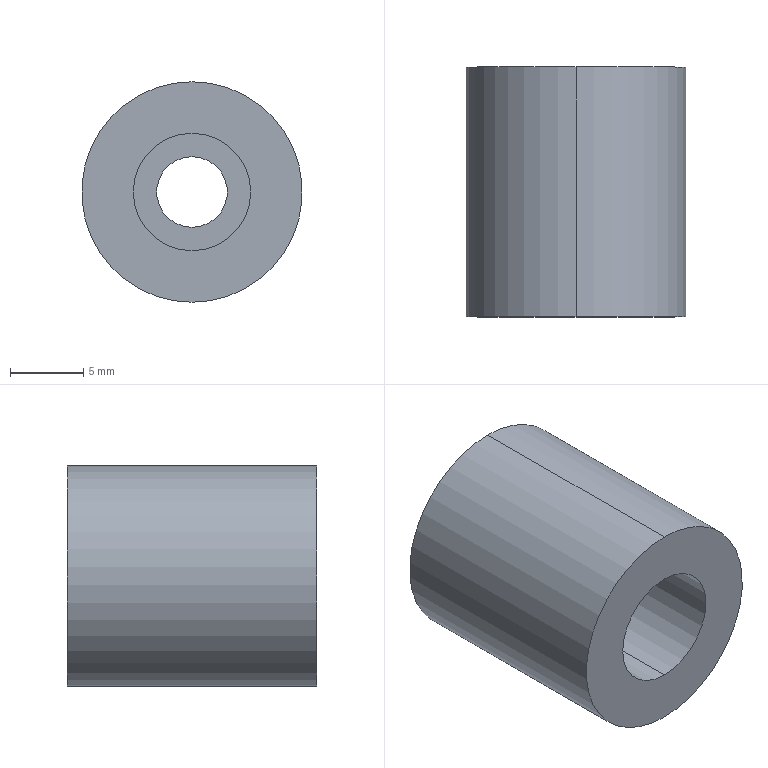Part | SolidWorks | features BaseBody 1 | 1 solid | 9 faces | box 15 x 17 x 15 mm | volume 2439 mm3 | cylinder 6 | plane 3 | commonest cylinder face diameters 4.8 x2 8 x2 15 x2
STEP:
#1=CARTESIAN_POINT('',(0.,17.,-7.5));
#2=VERTEX_POINT('',#1);
#3=CARTESIAN_POINT('',(0.,17.,7.5));
#4=VERTEX_POINT('',#3);
#5=CARTESIAN_POINT('',(0.,17.,0.));
#6=DIRECTION('',(0.,-1.,0.));
#7=DIRECTION('',(0.,0.,-1.));
#8=AXIS2_PLACEMENT_3D('',#5,#6,#7);
#9=CIRCLE('',#8,7.5);
#10=EDGE_CURVE('',#2,#4,#9,.T.);
#11=ORIENTED_EDGE('',*,*,#10,.T.);
#12=CARTESIAN_POINT('',(0.,0.,7.5));
#13=VERTEX_POINT('',#12);
#14=CARTESIAN_POINT('',(0.,17.,7.5));
#15=DIRECTION('',(0.,-1.,0.));
#16=VECTOR('',#15,1000.);
#17=LINE('',#14,#16);
#18=EDGE_CURVE('',#4,#13,#17,.T.);
#19=ORIENTED_EDGE('',*,*,#18,.T.);
#20=CARTESIAN_POINT('',(0.,0.,-7.5));
#21=VERTEX_POINT('',#20);
#22=CARTESIAN_POINT('',(0.,0.,0.));
#23=DIRECTION('',(0.,1.,0.));
#24=DIRECTION('',(0.,0.,-1.));
#25=AXIS2_PLACEMENT_3D('',#22,#23,#24);
#26=CIRCLE('',#25,7.5);
#27=EDGE_CURVE('',#13,#21,#26,.T.);
#28=ORIENTED_EDGE('',*,*,#27,.T.);
#29=CARTESIAN_POINT('',(0.,17.,-7.5));
#30=DIRECTION('',(0.,-1.,0.));
#31=VECTOR('',#30,1000.);
#32=LINE('',#29,#31);
#33=EDGE_CURVE('',#2,#21,#32,.T.);
#34=ORIENTED_EDGE('',*,*,#33,.F.);
#35=EDGE_LOOP('',(#11,#19,#28,#34));
#36=FACE_OUTER_BOUND('',#35,.T.);
#37=CARTESIAN_POINT('',(0.,17.,0.));
#38=DIRECTION('',(0.,-1.,0.));
#39=DIRECTION('',(0.,0.,-1.));
#40=AXIS2_PLACEMENT_3D('',#37,#38,#39);
#41=CYLINDRICAL_SURFACE('',#40,7.5);
#42=ADVANCED_FACE('',(#36),#41,.T.);
#43=CARTESIAN_POINT('',(0.,8.,4.));
#44=VERTEX_POINT('',#43);
#45=CARTESIAN_POINT('',(0.,8.,-4.));
#46=VERTEX_POINT('',#45);
#47=CARTESIAN_POINT('',(0.,8.,0.));
#48=DIRECTION('',(0.,-1.,0.));
#49=DIRECTION('',(0.,0.,-1.));
#50=AXIS2_PLACEMENT_3D('',#47,#48,#49);
#51=CIRCLE('',#50,4.);
#52=EDGE_CURVE('',#44,#46,#51,.T.);
#53=ORIENTED_EDGE('',*,*,#52,.F.);
#54=CARTESIAN_POINT('',(0.,0.,4.));
#55=VERTEX_POINT('',#54);
#56=CARTESIAN_POINT('',(0.,0.,4.));
#57=DIRECTION('',(0.,-1.,0.));
#58=VECTOR('',#57,1000.);
#59=LINE('',#56,#58);
#60=EDGE_CURVE('',#44,#55,#59,.T.);
#61=ORIENTED_EDGE('',*,*,#60,.T.);
#62=CARTESIAN_POINT('',(0.,0.,-4.));
#63=VERTEX_POINT('',#62);
#64=CARTESIAN_POINT('',(0.,0.,0.));
#65=DIRECTION('',(0.,-1.,0.));
#66=DIRECTION('',(0.,0.,-1.));
#67=AXIS2_PLACEMENT_3D('',#64,#65,#66);
#68=CIRCLE('',#67,4.);
#69=EDGE_CURVE('',#55,#63,#68,.T.);
#70=ORIENTED_EDGE('',*,*,#69,.T.);
#71=CARTESIAN_POINT('',(0.,0.,-4.));
#72=DIRECTION('',(0.,-1.,0.));
#73=VECTOR('',#72,1000.);
#74=LINE('',#71,#73);
#75=EDGE_CURVE('',#46,#63,#74,.T.);
#76=ORIENTED_EDGE('',*,*,#75,.F.);
#77=EDGE_LOOP('',(#53,#61,#70,#76));
#78=FACE_OUTER_BOUND('',#77,.T.);
#79=CARTESIAN_POINT('',(0.,0.,0.));
#80=DIRECTION('',(0.,-1.,0.));
#81=DIRECTION('',(0.,0.,-1.));
#82=AXIS2_PLACEMENT_3D('',#79,#80,#81);
#83=CYLINDRICAL_SURFACE('',#82,4.);
#84=ADVANCED_FACE('',(#78),#83,.F.);
#85=CARTESIAN_POINT('',(0.,17.,2.4));
#86=VERTEX_POINT('',#85);
#87=CARTESIAN_POINT('',(0.,17.,-2.4));
#88=VERTEX_POINT('',#87);
#89=CARTESIAN_POINT('',(0.,17.,0.));
#90=DIRECTION('',(0.,-1.,0.));
#91=DIRECTION('',(0.,0.,-1.));
#92=AXIS2_PLACEMENT_3D('',#89,#90,#91);
#93=CIRCLE('',#92,2.4);
#94=EDGE_CURVE('',#86,#88,#93,.T.);
#95=ORIENTED_EDGE('',*,*,#94,.F.);
#96=CARTESIAN_POINT('',(0.,8.,2.4));
#97=VERTEX_POINT('',#96);
#98=CARTESIAN_POINT('',(0.,0.,2.4));
#99=DIRECTION('',(0.,-1.,0.));
#100=VECTOR('',#99,1000.);
#101=LINE('',#98,#100);
#102=EDGE_CURVE('',#86,#97,#101,.T.);
#103=ORIENTED_EDGE('',*,*,#102,.T.);
#104=CARTESIAN_POINT('',(0.,8.,-2.4));
#105=VERTEX_POINT('',#104);
#106=CARTESIAN_POINT('',(0.,8.,0.));
#107=DIRECTION('',(0.,1.,0.));
#108=DIRECTION('',(0.,0.,-1.));
#109=AXIS2_PLACEMENT_3D('',#106,#107,#108);
#110=CIRCLE('',#109,2.4);
#111=EDGE_CURVE('',#105,#97,#110,.T.);
#112=ORIENTED_EDGE('',*,*,#111,.F.);
#113=CARTESIAN_POINT('',(0.,0.,-2.4));
#114=DIRECTION('',(0.,-1.,0.));
#115=VECTOR('',#114,1000.);
#116=LINE('',#113,#115);
#117=EDGE_CURVE('',#88,#105,#116,.T.);
#118=ORIENTED_EDGE('',*,*,#117,.F.);
#119=EDGE_LOOP('',(#95,#103,#112,#118));
#120=FACE_OUTER_BOUND('',#119,.T.);
#121=CARTESIAN_POINT('',(0.,0.,0.));
#122=DIRECTION('',(0.,-1.,0.));
#123=DIRECTION('',(0.,0.,-1.));
#124=AXIS2_PLACEMENT_3D('',#121,#122,#123);
#125=CYLINDRICAL_SURFACE('',#124,2.4);
#126=ADVANCED_FACE('',(#120),#125,.F.);
#127=ORIENTED_EDGE('',*,*,#18,.F.);
#128=CARTESIAN_POINT('',(0.,17.,0.));
#129=DIRECTION('',(0.,-1.,0.));
#130=DIRECTION('',(0.,0.,-1.));
#131=AXIS2_PLACEMENT_3D('',#128,#129,#130);
#132=CIRCLE('',#131,7.5);
#133=EDGE_CURVE('',#4,#2,#132,.T.);
#134=ORIENTED_EDGE('',*,*,#133,.T.);
#135=ORIENTED_EDGE('',*,*,#33,.T.);
#136=CARTESIAN_POINT('',(0.,0.,0.));
#137=DIRECTION('',(0.,1.,0.));
#138=DIRECTION('',(0.,0.,-1.));
#139=AXIS2_PLACEMENT_3D('',#136,#137,#138);
#140=CIRCLE('',#139,7.5);
#141=EDGE_CURVE('',#21,#13,#140,.T.);
#142=ORIENTED_EDGE('',*,*,#141,.T.);
#143=EDGE_LOOP('',(#127,#134,#135,#142));
#144=FACE_OUTER_BOUND('',#143,.T.);
#145=CARTESIAN_POINT('',(0.,17.,0.));
#146=DIRECTION('',(0.,-1.,0.));
#147=DIRECTION('',(0.,0.,-1.));
#148=AXIS2_PLACEMENT_3D('',#145,#146,#147);
#149=CYLINDRICAL_SURFACE('',#148,7.5);
#150=ADVANCED_FACE('',(#144),#149,.T.);
#151=ORIENTED_EDGE('',*,*,#141,.F.);
#152=ORIENTED_EDGE('',*,*,#27,.F.);
#153=EDGE_LOOP('',(#151,#152));
#154=FACE_OUTER_BOUND('',#153,.T.);
#155=CARTESIAN_POINT('',(0.,0.,0.));
#156=DIRECTION('',(0.,-1.,0.));
#157=DIRECTION('',(0.,0.,-1.));
#158=AXIS2_PLACEMENT_3D('',#155,#156,#157);
#159=CIRCLE('',#158,4.);
#160=EDGE_CURVE('',#63,#55,#159,.T.);
#161=ORIENTED_EDGE('',*,*,#160,.F.);
#162=ORIENTED_EDGE('',*,*,#69,.F.);
#163=EDGE_LOOP('',(#161,#162));
#164=FACE_BOUND('',#163,.T.);
#165=CARTESIAN_POINT('',(0.,0.,0.));
#166=DIRECTION('',(0.,1.,0.));
#167=DIRECTION('',(0.,0.,1.));
#168=AXIS2_PLACEMENT_3D('',#165,#166,#167);
#169=PLANE('',#168);
#170=ADVANCED_FACE('',(#154,#164),#169,.F.);
#171=ORIENTED_EDGE('',*,*,#10,.F.);
#172=ORIENTED_EDGE('',*,*,#133,.F.);
#173=EDGE_LOOP('',(#171,#172));
#174=FACE_OUTER_BOUND('',#173,.T.);
#175=CARTESIAN_POINT('',(0.,17.,0.));
#176=DIRECTION('',(0.,-1.,0.));
#177=DIRECTION('',(0.,0.,-1.));
#178=AXIS2_PLACEMENT_3D('',#175,#176,#177);
#179=CIRCLE('',#178,2.4);
#180=EDGE_CURVE('',#88,#86,#179,.T.);
#181=ORIENTED_EDGE('',*,*,#180,.T.);
#182=ORIENTED_EDGE('',*,*,#94,.T.);
#183=EDGE_LOOP('',(#181,#182));
#184=FACE_BOUND('',#183,.T.);
#185=CARTESIAN_POINT('',(0.,17.,0.));
#186=DIRECTION('',(0.,1.,0.));
#187=DIRECTION('',(0.,0.,1.));
#188=AXIS2_PLACEMENT_3D('',#185,#186,#187);
#189=PLANE('',#188);
#190=ADVANCED_FACE('',(#174,#184),#189,.T.);
#191=ORIENTED_EDGE('',*,*,#60,.F.);
#192=CARTESIAN_POINT('',(0.,8.,0.));
#193=DIRECTION('',(0.,-1.,0.));
#194=DIRECTION('',(0.,0.,-1.));
#195=AXIS2_PLACEMENT_3D('',#192,#193,#194);
#196=CIRCLE('',#195,4.);
#197=EDGE_CURVE('',#46,#44,#196,.T.);
#198=ORIENTED_EDGE('',*,*,#197,.F.);
#199=ORIENTED_EDGE('',*,*,#75,.T.);
#200=ORIENTED_EDGE('',*,*,#160,.T.);
#201=EDGE_LOOP('',(#191,#198,#199,#200));
#202=FACE_OUTER_BOUND('',#201,.T.);
#203=CARTESIAN_POINT('',(0.,0.,0.));
#204=DIRECTION('',(0.,-1.,0.));
#205=DIRECTION('',(0.,0.,-1.));
#206=AXIS2_PLACEMENT_3D('',#203,#204,#205);
#207=CYLINDRICAL_SURFACE('',#206,4.);
#208=ADVANCED_FACE('',(#202),#207,.F.);
#209=ORIENTED_EDGE('',*,*,#102,.F.);
#210=ORIENTED_EDGE('',*,*,#180,.F.);
#211=ORIENTED_EDGE('',*,*,#117,.T.);
#212=CARTESIAN_POINT('',(0.,8.,0.));
#213=DIRECTION('',(0.,1.,0.));
#214=DIRECTION('',(0.,0.,-1.));
#215=AXIS2_PLACEMENT_3D('',#212,#213,#214);
#216=CIRCLE('',#215,2.4);
#217=EDGE_CURVE('',#97,#105,#216,.T.);
#218=ORIENTED_EDGE('',*,*,#217,.F.);
#219=EDGE_LOOP('',(#209,#210,#211,#218));
#220=FACE_OUTER_BOUND('',#219,.T.);
#221=CARTESIAN_POINT('',(0.,0.,0.));
#222=DIRECTION('',(0.,-1.,0.));
#223=DIRECTION('',(0.,0.,-1.));
#224=AXIS2_PLACEMENT_3D('',#221,#222,#223);
#225=CYLINDRICAL_SURFACE('',#224,2.4);
#226=ADVANCED_FACE('',(#220),#225,.F.);
#227=ORIENTED_EDGE('',*,*,#197,.T.);
#228=ORIENTED_EDGE('',*,*,#52,.T.);
#229=EDGE_LOOP('',(#227,#228));
#230=FACE_OUTER_BOUND('',#229,.T.);
#231=ORIENTED_EDGE('',*,*,#111,.T.);
#232=ORIENTED_EDGE('',*,*,#217,.T.);
#233=EDGE_LOOP('',(#231,#232));
#234=FACE_BOUND('',#233,.T.);
#235=CARTESIAN_POINT('',(2.4,8.,0.));
#236=DIRECTION('',(0.,1.,0.));
#237=DIRECTION('',(0.,0.,1.));
#238=AXIS2_PLACEMENT_3D('',#235,#236,#237);
#239=PLANE('',#238);
#240=ADVANCED_FACE('',(#230,#234),#239,.F.);
#241=CLOSED_SHELL('',(#42,#84,#126,#150,#170,#190,#208,#226,#240));
#242=MANIFOLD_SOLID_BREP('',#241);
#243=CARTESIAN_POINT('',(0.,0.,0.));
#244=DIRECTION('',(0.,0.,1.));
#245=DIRECTION('',(1.,0.,0.));
#246=AXIS2_PLACEMENT_3D('',#243,#244,#245);
#247=(LENGTH_UNIT()NAMED_UNIT(*)SI_UNIT(.MILLI.,.METRE.));
#248=UNCERTAINTY_MEASURE_WITH_UNIT(LENGTH_MEASURE(0.00001),#247,'','');
#249=(NAMED_UNIT(*)PLANE_ANGLE_UNIT()SI_UNIT($,.RADIAN.));
#250=(NAMED_UNIT(*)SI_UNIT($,.STERADIAN.)SOLID_ANGLE_UNIT());
#251=(GEOMETRIC_REPRESENTATION_CONTEXT(3)GLOBAL_UNCERTAINTY_ASSIGNED_CONTEXT((#248))GLOBAL_UNIT_ASSIGNED_CONTEXT((#247,#249,#250))REPRESENTATION_CONTEXT('',''));
#252=ADVANCED_BREP_SHAPE_REPRESENTATION('',(#242,#246),#251);